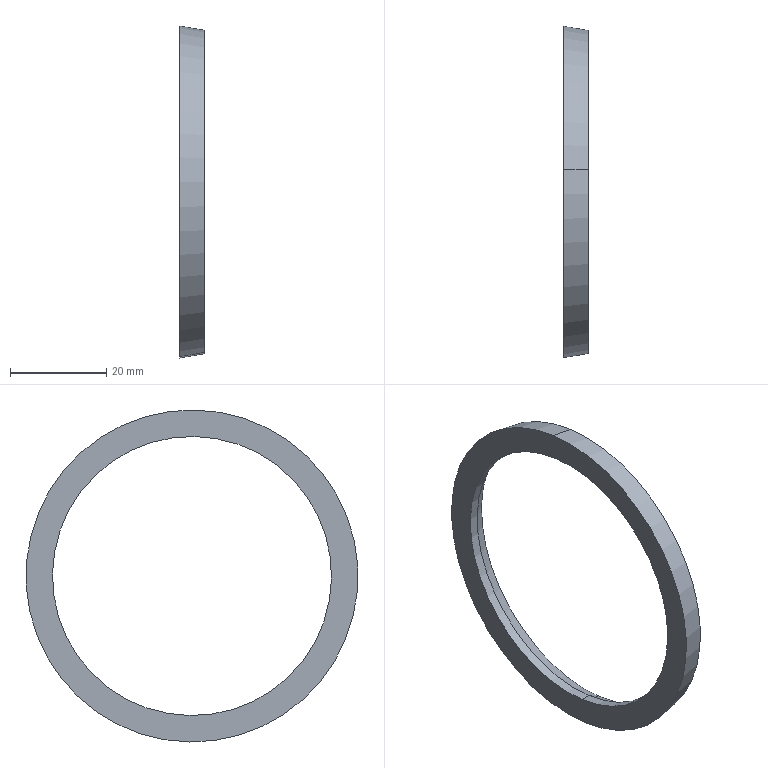Part | NX | features BREP 1 | 1 solid | 8 faces | box 5 x 69 x 69 mm | volume 4531 mm3 | cone 4 | cylinder 2 | plane 2 | commonest cylinder face diameters 58 x2
STEP:
#1=CARTESIAN_POINT('',(-56.922,3.913,28.735));
#2=VERTEX_POINT('',#1);
#3=CARTESIAN_POINT('',(-56.922,-3.913,-28.735));
#4=VERTEX_POINT('',#3);
#5=CARTESIAN_POINT('',(-56.922,0.,0.));
#6=DIRECTION('',(1.,0.,0.));
#7=DIRECTION('',(0.,-0.1349,-0.9909));
#8=AXIS2_PLACEMENT_3D('',#5,#6,#7);
#9=CIRCLE('',#8,29.);
#10=EDGE_CURVE('',#2,#4,#9,.T.);
#11=ORIENTED_EDGE('',*,*,#10,.F.);
#12=CARTESIAN_POINT('',(-53.925,4.146,30.449));
#13=VERTEX_POINT('',#12);
#14=CARTESIAN_POINT('',(-53.925,4.146,30.449));
#15=DIRECTION('',(0.866,0.06746,0.4954));
#16=VECTOR('',#15,1000.);
#17=LINE('',#14,#16);
#18=EDGE_CURVE('',#13,#2,#17,.F.);
#19=ORIENTED_EDGE('',*,*,#18,.F.);
#20=CARTESIAN_POINT('',(-53.925,-4.146,-30.449));
#21=VERTEX_POINT('',#20);
#22=CARTESIAN_POINT('',(-53.925,0.,0.));
#23=DIRECTION('',(-1.,0.,0.));
#24=DIRECTION('',(0.,-0.1349,-0.9909));
#25=AXIS2_PLACEMENT_3D('',#22,#23,#24);
#26=CIRCLE('',#25,30.73);
#27=EDGE_CURVE('',#21,#13,#26,.T.);
#28=ORIENTED_EDGE('',*,*,#27,.F.);
#29=CARTESIAN_POINT('',(-53.925,-4.146,-30.449));
#30=DIRECTION('',(0.866,-0.06746,-0.4954));
#31=VECTOR('',#30,1000.);
#32=LINE('',#29,#31);
#33=EDGE_CURVE('',#21,#4,#32,.F.);
#34=ORIENTED_EDGE('',*,*,#33,.T.);
#35=EDGE_LOOP('',(#11,#19,#28,#34));
#36=FACE_BOUND('',#35,.T.);
#37=CARTESIAN_POINT('',(-53.925,0.,0.));
#38=DIRECTION('',(1.,0.,0.));
#39=DIRECTION('',(0.,0.1349,0.9909));
#40=AXIS2_PLACEMENT_3D('',#37,#38,#39);
#41=CONICAL_SURFACE('',#40,30.73,0.5236);
#42=ADVANCED_FACE('',(#36),#41,.F.);
#43=ORIENTED_EDGE('',*,*,#10,.T.);
#44=CARTESIAN_POINT('',(-58.925,-3.913,-28.735));
#45=VERTEX_POINT('',#44);
#46=CARTESIAN_POINT('',(-530.465,-3.913,-28.735));
#47=DIRECTION('',(-1.,0.,0.));
#48=VECTOR('',#47,1000.);
#49=LINE('',#46,#48);
#50=EDGE_CURVE('',#4,#45,#49,.T.);
#51=ORIENTED_EDGE('',*,*,#50,.T.);
#52=CARTESIAN_POINT('',(-58.925,3.913,28.735));
#53=VERTEX_POINT('',#52);
#54=CARTESIAN_POINT('',(-58.925,0.,0.));
#55=DIRECTION('',(1.,0.,0.));
#56=DIRECTION('',(0.,-0.1349,-0.9909));
#57=AXIS2_PLACEMENT_3D('',#54,#55,#56);
#58=CIRCLE('',#57,29.);
#59=EDGE_CURVE('',#53,#45,#58,.T.);
#60=ORIENTED_EDGE('',*,*,#59,.F.);
#61=CARTESIAN_POINT('',(-530.465,3.913,28.735));
#62=DIRECTION('',(-1.,0.,0.));
#63=VECTOR('',#62,1000.);
#64=LINE('',#61,#63);
#65=EDGE_CURVE('',#2,#53,#64,.T.);
#66=ORIENTED_EDGE('',*,*,#65,.F.);
#67=EDGE_LOOP('',(#43,#51,#60,#66));
#68=FACE_BOUND('',#67,.T.);
#69=CARTESIAN_POINT('',(-530.465,0.,0.));
#70=DIRECTION('',(-1.,0.,0.));
#71=DIRECTION('',(0.,-0.1349,-0.9909));
#72=AXIS2_PLACEMENT_3D('',#69,#70,#71);
#73=CYLINDRICAL_SURFACE('',#72,29.);
#74=ADVANCED_FACE('',(#68),#73,.F.);
#75=CARTESIAN_POINT('',(-53.925,4.536,33.311));
#76=VERTEX_POINT('',#75);
#77=CARTESIAN_POINT('',(-53.925,-4.536,-33.311));
#78=VERTEX_POINT('',#77);
#79=CARTESIAN_POINT('',(-53.925,0.,0.));
#80=DIRECTION('',(1.,0.,0.));
#81=DIRECTION('',(0.,-0.1349,-0.9909));
#82=AXIS2_PLACEMENT_3D('',#79,#80,#81);
#83=CIRCLE('',#82,33.618);
#84=EDGE_CURVE('',#76,#78,#83,.T.);
#85=ORIENTED_EDGE('',*,*,#84,.F.);
#86=CARTESIAN_POINT('',(-58.925,4.655,34.185));
#87=VERTEX_POINT('',#86);
#88=CARTESIAN_POINT('',(-58.925,4.655,34.185));
#89=DIRECTION('',(-0.9848,0.02343,0.1721));
#90=VECTOR('',#89,1000.);
#91=LINE('',#88,#90);
#92=EDGE_CURVE('',#87,#76,#91,.F.);
#93=ORIENTED_EDGE('',*,*,#92,.F.);
#94=CARTESIAN_POINT('',(-58.925,-4.655,-34.185));
#95=VERTEX_POINT('',#94);
#96=CARTESIAN_POINT('',(-58.925,0.,0.));
#97=DIRECTION('',(1.,0.,0.));
#98=DIRECTION('',(0.,-0.1349,-0.9909));
#99=AXIS2_PLACEMENT_3D('',#96,#97,#98);
#100=CIRCLE('',#99,34.5);
#101=EDGE_CURVE('',#87,#95,#100,.T.);
#102=ORIENTED_EDGE('',*,*,#101,.T.);
#103=CARTESIAN_POINT('',(-58.925,-4.655,-34.185));
#104=DIRECTION('',(-0.9848,-0.02343,-0.1721));
#105=VECTOR('',#104,1000.);
#106=LINE('',#103,#105);
#107=EDGE_CURVE('',#95,#78,#106,.F.);
#108=ORIENTED_EDGE('',*,*,#107,.T.);
#109=EDGE_LOOP('',(#85,#93,#102,#108));
#110=FACE_BOUND('',#109,.T.);
#111=CARTESIAN_POINT('',(-58.925,0.,0.));
#112=DIRECTION('',(-1.,0.,0.));
#113=DIRECTION('',(0.,0.1349,0.9909));
#114=AXIS2_PLACEMENT_3D('',#111,#112,#113);
#115=CONICAL_SURFACE('',#114,34.5,0.1745);
#116=ADVANCED_FACE('',(#110),#115,.T.);
#117=ORIENTED_EDGE('',*,*,#92,.T.);
#118=CARTESIAN_POINT('',(-53.925,0.,0.));
#119=DIRECTION('',(1.,0.,0.));
#120=DIRECTION('',(0.,-0.1349,-0.9909));
#121=AXIS2_PLACEMENT_3D('',#118,#119,#120);
#122=CIRCLE('',#121,33.618);
#123=EDGE_CURVE('',#78,#76,#122,.T.);
#124=ORIENTED_EDGE('',*,*,#123,.F.);
#125=ORIENTED_EDGE('',*,*,#107,.F.);
#126=CARTESIAN_POINT('',(-58.925,0.,0.));
#127=DIRECTION('',(1.,0.,0.));
#128=DIRECTION('',(0.,-0.1349,-0.9909));
#129=AXIS2_PLACEMENT_3D('',#126,#127,#128);
#130=CIRCLE('',#129,34.5);
#131=EDGE_CURVE('',#95,#87,#130,.T.);
#132=ORIENTED_EDGE('',*,*,#131,.T.);
#133=EDGE_LOOP('',(#117,#124,#125,#132));
#134=FACE_BOUND('',#133,.T.);
#135=CARTESIAN_POINT('',(-58.925,0.,0.));
#136=DIRECTION('',(-1.,0.,0.));
#137=DIRECTION('',(0.,0.1349,0.9909));
#138=AXIS2_PLACEMENT_3D('',#135,#136,#137);
#139=CONICAL_SURFACE('',#138,34.5,0.1745);
#140=ADVANCED_FACE('',(#134),#139,.T.);
#141=ORIENTED_EDGE('',*,*,#27,.T.);
#142=CARTESIAN_POINT('',(-53.925,0.,0.));
#143=DIRECTION('',(-1.,0.,0.));
#144=DIRECTION('',(0.,-0.1349,-0.9909));
#145=AXIS2_PLACEMENT_3D('',#142,#143,#144);
#146=CIRCLE('',#145,30.73);
#147=EDGE_CURVE('',#13,#21,#146,.T.);
#148=ORIENTED_EDGE('',*,*,#147,.T.);
#149=EDGE_LOOP('',(#141,#148));
#150=FACE_BOUND('',#149,.T.);
#151=ORIENTED_EDGE('',*,*,#123,.T.);
#152=ORIENTED_EDGE('',*,*,#84,.T.);
#153=EDGE_LOOP('',(#151,#152));
#154=FACE_BOUND('',#153,.T.);
#155=CARTESIAN_POINT('',(-53.925,0.,0.));
#156=DIRECTION('',(1.,0.,0.));
#157=DIRECTION('',(0.,0.1349,0.9909));
#158=AXIS2_PLACEMENT_3D('',#155,#156,#157);
#159=PLANE('',#158);
#160=ADVANCED_FACE('',(#150,#154),#159,.T.);
#161=ORIENTED_EDGE('',*,*,#59,.T.);
#162=CARTESIAN_POINT('',(-58.925,0.,0.));
#163=DIRECTION('',(1.,0.,0.));
#164=DIRECTION('',(0.,-0.1349,-0.9909));
#165=AXIS2_PLACEMENT_3D('',#162,#163,#164);
#166=CIRCLE('',#165,29.);
#167=EDGE_CURVE('',#45,#53,#166,.T.);
#168=ORIENTED_EDGE('',*,*,#167,.T.);
#169=EDGE_LOOP('',(#161,#168));
#170=FACE_BOUND('',#169,.T.);
#171=ORIENTED_EDGE('',*,*,#131,.F.);
#172=ORIENTED_EDGE('',*,*,#101,.F.);
#173=EDGE_LOOP('',(#171,#172));
#174=FACE_BOUND('',#173,.T.);
#175=CARTESIAN_POINT('',(-58.925,0.,0.));
#176=DIRECTION('',(1.,0.,0.));
#177=DIRECTION('',(0.,0.1349,0.9909));
#178=AXIS2_PLACEMENT_3D('',#175,#176,#177);
#179=PLANE('',#178);
#180=ADVANCED_FACE('',(#170,#174),#179,.F.);
#181=ORIENTED_EDGE('',*,*,#50,.F.);
#182=CARTESIAN_POINT('',(-56.922,0.,0.));
#183=DIRECTION('',(1.,0.,0.));
#184=DIRECTION('',(0.,-0.1349,-0.9909));
#185=AXIS2_PLACEMENT_3D('',#182,#183,#184);
#186=CIRCLE('',#185,29.);
#187=EDGE_CURVE('',#4,#2,#186,.T.);
#188=ORIENTED_EDGE('',*,*,#187,.T.);
#189=ORIENTED_EDGE('',*,*,#65,.T.);
#190=ORIENTED_EDGE('',*,*,#167,.F.);
#191=EDGE_LOOP('',(#181,#188,#189,#190));
#192=FACE_BOUND('',#191,.T.);
#193=CARTESIAN_POINT('',(-530.465,0.,0.));
#194=DIRECTION('',(-1.,0.,0.));
#195=DIRECTION('',(0.,-0.1349,-0.9909));
#196=AXIS2_PLACEMENT_3D('',#193,#194,#195);
#197=CYLINDRICAL_SURFACE('',#196,29.);
#198=ADVANCED_FACE('',(#192),#197,.F.);
#199=ORIENTED_EDGE('',*,*,#18,.T.);
#200=ORIENTED_EDGE('',*,*,#187,.F.);
#201=ORIENTED_EDGE('',*,*,#33,.F.);
#202=ORIENTED_EDGE('',*,*,#147,.F.);
#203=EDGE_LOOP('',(#199,#200,#201,#202));
#204=FACE_BOUND('',#203,.T.);
#205=CARTESIAN_POINT('',(-53.925,0.,0.));
#206=DIRECTION('',(1.,0.,0.));
#207=DIRECTION('',(0.,0.1349,0.9909));
#208=AXIS2_PLACEMENT_3D('',#205,#206,#207);
#209=CONICAL_SURFACE('',#208,30.73,0.5236);
#210=ADVANCED_FACE('',(#204),#209,.F.);
#211=CLOSED_SHELL('',(#42,#74,#116,#140,#160,#180,#198,#210));
#212=MANIFOLD_SOLID_BREP('',#211);
#213=(LENGTH_UNIT()NAMED_UNIT(*)SI_UNIT(.MILLI.,.METRE.));
#214=UNCERTAINTY_MEASURE_WITH_UNIT(LENGTH_MEASURE(0.00001),#213,'','');
#215=(NAMED_UNIT(*)PLANE_ANGLE_UNIT()SI_UNIT($,.RADIAN.));
#216=(NAMED_UNIT(*)SI_UNIT($,.STERADIAN.)SOLID_ANGLE_UNIT());
#217=(GEOMETRIC_REPRESENTATION_CONTEXT(3)GLOBAL_UNCERTAINTY_ASSIGNED_CONTEXT((#214))GLOBAL_UNIT_ASSIGNED_CONTEXT((#213,#215,#216))REPRESENTATION_CONTEXT('',''));
#218=ADVANCED_BREP_SHAPE_REPRESENTATION('',(#212),#217);